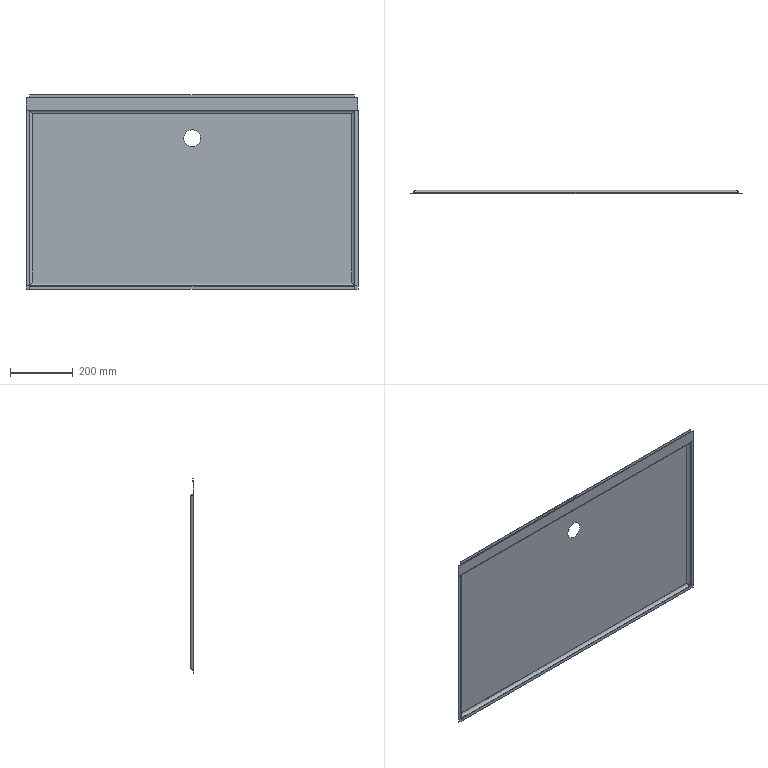Part | SolidWorks | features EdgeFlange 4, SMWeldBead 2, FlatPattern 1, ICE 1, SMBaseFlange 1, SheetMetal 1 | 1 solid | 118 faces | box 1058 x 10.6 x 620.2 mm | volume 404169 mm3 | plane 68 | cylinder 32 | spline 18 | commonest cylinder face diameters 0.2 x12 1.4 x10 18 x4 19.2 x4 54 x2